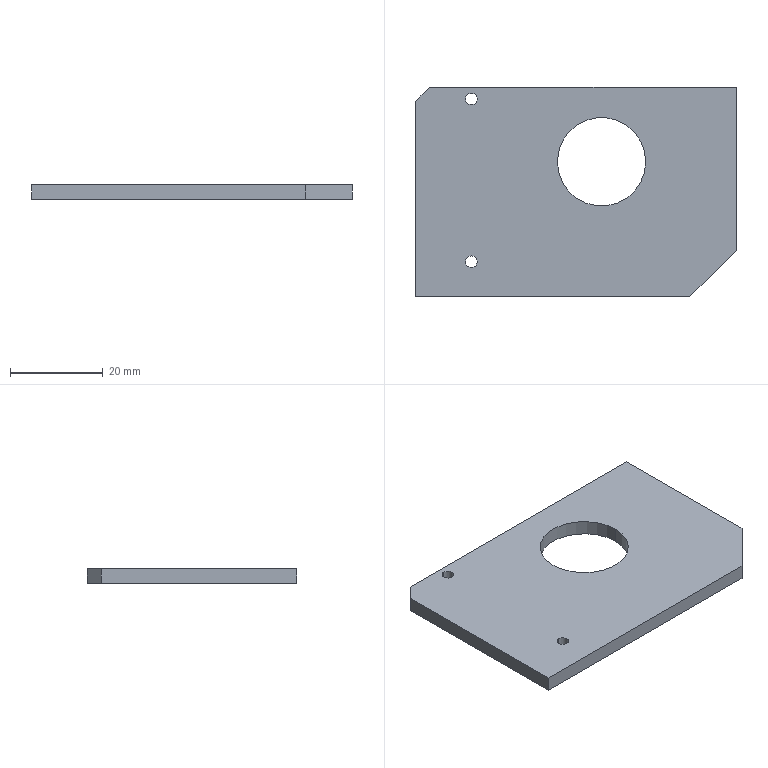Part | STEP file | [02]-14 | 1 solid | 14 faces | box 69 x 45 x 3.2 mm | volume 8823 mm3 | plane 8 | cylinder 6 | commonest cylinder face diameters 2.5 x4 19 x2
STEP:
#1=CARTESIAN_POINT('',(0.,0.,0.));
#2=DIRECTION('',(0.,0.,1.));
#3=DIRECTION('',(1.,0.,0.));
#4=AXIS2_PLACEMENT_3D('',#1,#2,#3);
#5=CARTESIAN_POINT('',(12.,-38.75,3.));
#6=VERTEX_POINT('',#5);
#7=CARTESIAN_POINT('',(12.,-38.75,-0.2));
#8=VERTEX_POINT('',#7);
#9=CARTESIAN_POINT('',(12.,-38.75,3.));
#10=DIRECTION('',(0.,0.,-1.));
#11=VECTOR('',#10,1.);
#12=LINE('',#9,#11);
#13=CARTESIAN_POINT('',(12.,-37.5,3.));
#14=DIRECTION('',(0.,0.,-1.));
#15=DIRECTION('',(0.,-1.,0.));
#16=AXIS2_PLACEMENT_3D('',#13,#14,#15);
#17=CYLINDRICAL_SURFACE('',#16,1.25);
#18=CARTESIAN_POINT('',(6.283,0.));
#19=DIRECTION('',(0.,1.));
#20=VECTOR('',#19,1.);
#21=LINE('',#18,#20);
#22=(GEOMETRIC_REPRESENTATION_CONTEXT(2)PARAMETRIC_REPRESENTATION_CONTEXT()REPRESENTATION_CONTEXT('',''));
#23=DEFINITIONAL_REPRESENTATION('',(#21),#22);
#24=PCURVE('',#17,#23);
#25=CARTESIAN_POINT('',(12.,-37.5,3.));
#26=DIRECTION('',(0.,0.,-1.));
#27=DIRECTION('',(0.,-1.,0.));
#28=AXIS2_PLACEMENT_3D('',#25,#26,#27);
#29=CYLINDRICAL_SURFACE('',#28,1.25);
#30=CARTESIAN_POINT('',(0.,0.));
#31=DIRECTION('',(0.,1.));
#32=VECTOR('',#31,1.);
#33=LINE('',#30,#32);
#34=(GEOMETRIC_REPRESENTATION_CONTEXT(2)PARAMETRIC_REPRESENTATION_CONTEXT()REPRESENTATION_CONTEXT('',''));
#35=DEFINITIONAL_REPRESENTATION('',(#33),#34);
#36=PCURVE('',#29,#35);
#37=SURFACE_CURVE('',#12,(#24,#36),.PCURVE_S1.);
#38=EDGE_CURVE('',#6,#8,#37,.T.);
#39=ORIENTED_EDGE('',*,*,#38,.T.);
#40=CARTESIAN_POINT('',(12.,-36.25,-0.2));
#41=VERTEX_POINT('',#40);
#42=CARTESIAN_POINT('',(12.,-37.5,-0.2));
#43=DIRECTION('',(0.,0.,1.));
#44=DIRECTION('',(0.,1.,0.));
#45=AXIS2_PLACEMENT_3D('',#42,#43,#44);
#46=CIRCLE('',#45,1.25);
#47=CARTESIAN_POINT('',(9.425,3.2));
#48=DIRECTION('',(-1.,0.));
#49=VECTOR('',#48,1.);
#50=LINE('',#47,#49);
#51=(GEOMETRIC_REPRESENTATION_CONTEXT(2)PARAMETRIC_REPRESENTATION_CONTEXT()REPRESENTATION_CONTEXT('',''));
#52=DEFINITIONAL_REPRESENTATION('',(#50),#51);
#53=PCURVE('',#17,#52);
#54=CARTESIAN_POINT('',(34.5,-22.5,-0.2));
#55=DIRECTION('',(0.,0.,-1.));
#56=DIRECTION('',(0.,-1.,0.));
#57=AXIS2_PLACEMENT_3D('',#54,#55,#56);
#58=PLANE('',#57);
#59=CARTESIAN_POINT('',(13.75,22.5));
#60=CARTESIAN_POINT('',(13.75,24.665));
#61=CARTESIAN_POINT('',(15.625,23.583));
#62=CARTESIAN_POINT('',(17.5,22.5));
#63=CARTESIAN_POINT('',(15.625,21.417));
#64=CARTESIAN_POINT('',(13.75,20.335));
#65=CARTESIAN_POINT('',(13.75,22.5));
#66=(BOUNDED_CURVE()B_SPLINE_CURVE(2,(#59,#60,#61,#62,#63,#64,#65),.UNSPECIFIED.,.T.,.F.)B_SPLINE_CURVE_WITH_KNOTS((1,2,2,2,2,1),(-2.094,0.,2.094,4.189,6.283,8.378),.UNSPECIFIED.)CURVE()GEOMETRIC_REPRESENTATION_ITEM()RATIONAL_B_SPLINE_CURVE((1.,0.5,1.,0.5,1.,0.5,1.))REPRESENTATION_ITEM(''));
#67=(GEOMETRIC_REPRESENTATION_CONTEXT(2)PARAMETRIC_REPRESENTATION_CONTEXT()REPRESENTATION_CONTEXT('',''));
#68=DEFINITIONAL_REPRESENTATION('',(#66),#67);
#69=PCURVE('',#58,#68);
#70=SURFACE_CURVE('',#46,(#53,#69),.PCURVE_S1.);
#71=EDGE_CURVE('',#8,#41,#70,.T.);
#72=ORIENTED_EDGE('',*,*,#71,.T.);
#73=CARTESIAN_POINT('',(12.,-36.25,3.));
#74=VERTEX_POINT('',#73);
#75=CARTESIAN_POINT('',(12.,-36.25,3.));
#76=DIRECTION('',(0.,0.,-1.));
#77=VECTOR('',#76,1.);
#78=LINE('',#75,#77);
#79=CARTESIAN_POINT('',(3.142,0.));
#80=DIRECTION('',(0.,1.));
#81=VECTOR('',#80,1.);
#82=LINE('',#79,#81);
#83=(GEOMETRIC_REPRESENTATION_CONTEXT(2)PARAMETRIC_REPRESENTATION_CONTEXT()REPRESENTATION_CONTEXT('',''));
#84=DEFINITIONAL_REPRESENTATION('',(#82),#83);
#85=PCURVE('',#17,#84);
#86=CARTESIAN_POINT('',(3.142,0.));
#87=DIRECTION('',(0.,1.));
#88=VECTOR('',#87,1.);
#89=LINE('',#86,#88);
#90=(GEOMETRIC_REPRESENTATION_CONTEXT(2)PARAMETRIC_REPRESENTATION_CONTEXT()REPRESENTATION_CONTEXT('',''));
#91=DEFINITIONAL_REPRESENTATION('',(#89),#90);
#92=PCURVE('',#29,#91);
#93=SURFACE_CURVE('',#78,(#85,#92),.PCURVE_S1.);
#94=EDGE_CURVE('',#74,#41,#93,.T.);
#95=ORIENTED_EDGE('',*,*,#94,.F.);
#96=CARTESIAN_POINT('',(12.,-37.5,3.));
#97=DIRECTION('',(0.,0.,-1.));
#98=DIRECTION('',(0.,-1.,0.));
#99=AXIS2_PLACEMENT_3D('',#96,#97,#98);
#100=CIRCLE('',#99,1.25);
#101=CARTESIAN_POINT('',(0.,0.));
#102=DIRECTION('',(1.,0.));
#103=VECTOR('',#102,1.);
#104=LINE('',#101,#103);
#105=(GEOMETRIC_REPRESENTATION_CONTEXT(2)PARAMETRIC_REPRESENTATION_CONTEXT()REPRESENTATION_CONTEXT('',''));
#106=DEFINITIONAL_REPRESENTATION('',(#104),#105);
#107=PCURVE('',#17,#106);
#108=CARTESIAN_POINT('',(34.5,-22.5,3.));
#109=DIRECTION('',(0.,0.,1.));
#110=DIRECTION('',(0.,1.,0.));
#111=AXIS2_PLACEMENT_3D('',#108,#109,#110);
#112=PLANE('',#111);
#113=CARTESIAN_POINT('',(-16.25,22.5));
#114=CARTESIAN_POINT('',(-16.25,24.665));
#115=CARTESIAN_POINT('',(-14.375,23.583));
#116=CARTESIAN_POINT('',(-12.5,22.5));
#117=CARTESIAN_POINT('',(-14.375,21.417));
#118=CARTESIAN_POINT('',(-16.25,20.335));
#119=CARTESIAN_POINT('',(-16.25,22.5));
#120=(BOUNDED_CURVE()B_SPLINE_CURVE(2,(#113,#114,#115,#116,#117,#118,#119),.UNSPECIFIED.,.T.,.F.)B_SPLINE_CURVE_WITH_KNOTS((1,2,2,2,2,1),(-2.094,0.,2.094,4.189,6.283,8.378),.UNSPECIFIED.)CURVE()GEOMETRIC_REPRESENTATION_ITEM()RATIONAL_B_SPLINE_CURVE((1.,0.5,1.,0.5,1.,0.5,1.))REPRESENTATION_ITEM(''));
#121=(GEOMETRIC_REPRESENTATION_CONTEXT(2)PARAMETRIC_REPRESENTATION_CONTEXT()REPRESENTATION_CONTEXT('',''));
#122=DEFINITIONAL_REPRESENTATION('',(#120),#121);
#123=PCURVE('',#112,#122);
#124=SURFACE_CURVE('',#100,(#107,#123),.PCURVE_S1.);
#125=EDGE_CURVE('',#74,#6,#124,.T.);
#126=ORIENTED_EDGE('',*,*,#125,.T.);
#127=EDGE_LOOP('',(#39,#72,#95,#126));
#128=FACE_BOUND('',#127,.F.);
#129=ADVANCED_FACE('',(#128),#17,.F.);
#130=CARTESIAN_POINT('',(12.,-3.75,3.));
#131=VERTEX_POINT('',#130);
#132=CARTESIAN_POINT('',(12.,-3.75,-0.2));
#133=VERTEX_POINT('',#132);
#134=CARTESIAN_POINT('',(12.,-3.75,3.));
#135=DIRECTION('',(0.,0.,-1.));
#136=VECTOR('',#135,1.);
#137=LINE('',#134,#136);
#138=CARTESIAN_POINT('',(12.,-2.5,3.));
#139=DIRECTION('',(0.,0.,-1.));
#140=DIRECTION('',(0.,-1.,0.));
#141=AXIS2_PLACEMENT_3D('',#138,#139,#140);
#142=CYLINDRICAL_SURFACE('',#141,1.25);
#143=CARTESIAN_POINT('',(6.283,0.));
#144=DIRECTION('',(0.,1.));
#145=VECTOR('',#144,1.);
#146=LINE('',#143,#145);
#147=(GEOMETRIC_REPRESENTATION_CONTEXT(2)PARAMETRIC_REPRESENTATION_CONTEXT()REPRESENTATION_CONTEXT('',''));
#148=DEFINITIONAL_REPRESENTATION('',(#146),#147);
#149=PCURVE('',#142,#148);
#150=CARTESIAN_POINT('',(12.,-2.5,3.));
#151=DIRECTION('',(0.,0.,-1.));
#152=DIRECTION('',(0.,-1.,0.));
#153=AXIS2_PLACEMENT_3D('',#150,#151,#152);
#154=CYLINDRICAL_SURFACE('',#153,1.25);
#155=CARTESIAN_POINT('',(0.,0.));
#156=DIRECTION('',(0.,1.));
#157=VECTOR('',#156,1.);
#158=LINE('',#155,#157);
#159=(GEOMETRIC_REPRESENTATION_CONTEXT(2)PARAMETRIC_REPRESENTATION_CONTEXT()REPRESENTATION_CONTEXT('',''));
#160=DEFINITIONAL_REPRESENTATION('',(#158),#159);
#161=PCURVE('',#154,#160);
#162=SURFACE_CURVE('',#137,(#149,#161),.PCURVE_S1.);
#163=EDGE_CURVE('',#131,#133,#162,.T.);
#164=ORIENTED_EDGE('',*,*,#163,.T.);
#165=CARTESIAN_POINT('',(12.,-1.25,-0.2));
#166=VERTEX_POINT('',#165);
#167=CARTESIAN_POINT('',(12.,-2.5,-0.2));
#168=DIRECTION('',(0.,0.,1.));
#169=DIRECTION('',(0.,1.,0.));
#170=AXIS2_PLACEMENT_3D('',#167,#168,#169);
#171=CIRCLE('',#170,1.25);
#172=CARTESIAN_POINT('',(9.425,3.2));
#173=DIRECTION('',(-1.,0.));
#174=VECTOR('',#173,1.);
#175=LINE('',#172,#174);
#176=(GEOMETRIC_REPRESENTATION_CONTEXT(2)PARAMETRIC_REPRESENTATION_CONTEXT()REPRESENTATION_CONTEXT('',''));
#177=DEFINITIONAL_REPRESENTATION('',(#175),#176);
#178=PCURVE('',#142,#177);
#179=CARTESIAN_POINT('',(-21.25,22.5));
#180=CARTESIAN_POINT('',(-21.25,24.665));
#181=CARTESIAN_POINT('',(-19.375,23.583));
#182=CARTESIAN_POINT('',(-17.5,22.5));
#183=CARTESIAN_POINT('',(-19.375,21.417));
#184=CARTESIAN_POINT('',(-21.25,20.335));
#185=CARTESIAN_POINT('',(-21.25,22.5));
#186=(BOUNDED_CURVE()B_SPLINE_CURVE(2,(#179,#180,#181,#182,#183,#184,#185),.UNSPECIFIED.,.T.,.F.)B_SPLINE_CURVE_WITH_KNOTS((1,2,2,2,2,1),(-2.094,0.,2.094,4.189,6.283,8.378),.UNSPECIFIED.)CURVE()GEOMETRIC_REPRESENTATION_ITEM()RATIONAL_B_SPLINE_CURVE((1.,0.5,1.,0.5,1.,0.5,1.))REPRESENTATION_ITEM(''));
#187=(GEOMETRIC_REPRESENTATION_CONTEXT(2)PARAMETRIC_REPRESENTATION_CONTEXT()REPRESENTATION_CONTEXT('',''));
#188=DEFINITIONAL_REPRESENTATION('',(#186),#187);
#189=PCURVE('',#58,#188);
#190=SURFACE_CURVE('',#171,(#178,#189),.PCURVE_S1.);
#191=EDGE_CURVE('',#133,#166,#190,.T.);
#192=ORIENTED_EDGE('',*,*,#191,.T.);
#193=CARTESIAN_POINT('',(12.,-1.25,3.));
#194=VERTEX_POINT('',#193);
#195=CARTESIAN_POINT('',(12.,-1.25,3.));
#196=DIRECTION('',(0.,0.,-1.));
#197=VECTOR('',#196,1.);
#198=LINE('',#195,#197);
#199=CARTESIAN_POINT('',(3.142,0.));
#200=DIRECTION('',(0.,1.));
#201=VECTOR('',#200,1.);
#202=LINE('',#199,#201);
#203=(GEOMETRIC_REPRESENTATION_CONTEXT(2)PARAMETRIC_REPRESENTATION_CONTEXT()REPRESENTATION_CONTEXT('',''));
#204=DEFINITIONAL_REPRESENTATION('',(#202),#203);
#205=PCURVE('',#142,#204);
#206=CARTESIAN_POINT('',(3.142,0.));
#207=DIRECTION('',(0.,1.));
#208=VECTOR('',#207,1.);
#209=LINE('',#206,#208);
#210=(GEOMETRIC_REPRESENTATION_CONTEXT(2)PARAMETRIC_REPRESENTATION_CONTEXT()REPRESENTATION_CONTEXT('',''));
#211=DEFINITIONAL_REPRESENTATION('',(#209),#210);
#212=PCURVE('',#154,#211);
#213=SURFACE_CURVE('',#198,(#205,#212),.PCURVE_S1.);
#214=EDGE_CURVE('',#194,#166,#213,.T.);
#215=ORIENTED_EDGE('',*,*,#214,.F.);
#216=CARTESIAN_POINT('',(12.,-2.5,3.));
#217=DIRECTION('',(0.,0.,-1.));
#218=DIRECTION('',(0.,-1.,0.));
#219=AXIS2_PLACEMENT_3D('',#216,#217,#218);
#220=CIRCLE('',#219,1.25);
#221=CARTESIAN_POINT('',(0.,0.));
#222=DIRECTION('',(1.,0.));
#223=VECTOR('',#222,1.);
#224=LINE('',#221,#223);
#225=(GEOMETRIC_REPRESENTATION_CONTEXT(2)PARAMETRIC_REPRESENTATION_CONTEXT()REPRESENTATION_CONTEXT('',''));
#226=DEFINITIONAL_REPRESENTATION('',(#224),#225);
#227=PCURVE('',#142,#226);
#228=CARTESIAN_POINT('',(18.75,22.5));
#229=CARTESIAN_POINT('',(18.75,24.665));
#230=CARTESIAN_POINT('',(20.625,23.583));
#231=CARTESIAN_POINT('',(22.5,22.5));
#232=CARTESIAN_POINT('',(20.625,21.417));
#233=CARTESIAN_POINT('',(18.75,20.335));
#234=CARTESIAN_POINT('',(18.75,22.5));
#235=(BOUNDED_CURVE()B_SPLINE_CURVE(2,(#228,#229,#230,#231,#232,#233,#234),.UNSPECIFIED.,.T.,.F.)B_SPLINE_CURVE_WITH_KNOTS((1,2,2,2,2,1),(-2.094,0.,2.094,4.189,6.283,8.378),.UNSPECIFIED.)CURVE()GEOMETRIC_REPRESENTATION_ITEM()RATIONAL_B_SPLINE_CURVE((1.,0.5,1.,0.5,1.,0.5,1.))REPRESENTATION_ITEM(''));
#236=(GEOMETRIC_REPRESENTATION_CONTEXT(2)PARAMETRIC_REPRESENTATION_CONTEXT()REPRESENTATION_CONTEXT('',''));
#237=DEFINITIONAL_REPRESENTATION('',(#235),#236);
#238=PCURVE('',#112,#237);
#239=SURFACE_CURVE('',#220,(#227,#238),.PCURVE_S1.);
#240=EDGE_CURVE('',#194,#131,#239,.T.);
#241=ORIENTED_EDGE('',*,*,#240,.T.);
#242=EDGE_LOOP('',(#164,#192,#215,#241));
#243=FACE_BOUND('',#242,.F.);
#244=ADVANCED_FACE('',(#243),#142,.F.);
#245=CARTESIAN_POINT('',(49.5,-16.,-0.2));
#246=VERTEX_POINT('',#245);
#247=CARTESIAN_POINT('',(49.5,-16.,3.));
#248=VERTEX_POINT('',#247);
#249=CARTESIAN_POINT('',(49.5,-16.,-0.2));
#250=DIRECTION('',(0.,0.,1.));
#251=VECTOR('',#250,1.);
#252=LINE('',#249,#251);
#253=CARTESIAN_POINT('',(40.,-16.,-0.2));
#254=DIRECTION('',(0.,0.,1.));
#255=DIRECTION('',(1.,0.,0.));
#256=AXIS2_PLACEMENT_3D('',#253,#254,#255);
#257=CYLINDRICAL_SURFACE('',#256,9.5);
#258=CARTESIAN_POINT('',(6.283,0.));
#259=DIRECTION('',(0.,1.));
#260=VECTOR('',#259,1.);
#261=LINE('',#258,#260);
#262=(GEOMETRIC_REPRESENTATION_CONTEXT(2)PARAMETRIC_REPRESENTATION_CONTEXT()REPRESENTATION_CONTEXT('',''));
#263=DEFINITIONAL_REPRESENTATION('',(#261),#262);
#264=PCURVE('',#257,#263);
#265=CARTESIAN_POINT('',(40.,-16.,-0.2));
#266=DIRECTION('',(0.,0.,1.));
#267=DIRECTION('',(1.,0.,0.));
#268=AXIS2_PLACEMENT_3D('',#265,#266,#267);
#269=CYLINDRICAL_SURFACE('',#268,9.5);
#270=CARTESIAN_POINT('',(0.,0.));
#271=DIRECTION('',(0.,1.));
#272=VECTOR('',#271,1.);
#273=LINE('',#270,#272);
#274=(GEOMETRIC_REPRESENTATION_CONTEXT(2)PARAMETRIC_REPRESENTATION_CONTEXT()REPRESENTATION_CONTEXT('',''));
#275=DEFINITIONAL_REPRESENTATION('',(#273),#274);
#276=PCURVE('',#269,#275);
#277=SURFACE_CURVE('',#252,(#264,#276),.PCURVE_S1.);
#278=EDGE_CURVE('',#246,#248,#277,.T.);
#279=ORIENTED_EDGE('',*,*,#278,.T.);
#280=CARTESIAN_POINT('',(30.5,-16.,3.));
#281=VERTEX_POINT('',#280);
#282=CARTESIAN_POINT('',(40.,-16.,3.));
#283=DIRECTION('',(0.,0.,1.));
#284=DIRECTION('',(-1.,0.,0.));
#285=AXIS2_PLACEMENT_3D('',#282,#283,#284);
#286=CIRCLE('',#285,9.5);
#287=CARTESIAN_POINT('',(3.142,3.2));
#288=DIRECTION('',(1.,0.));
#289=VECTOR('',#288,1.);
#290=LINE('',#287,#289);
#291=(GEOMETRIC_REPRESENTATION_CONTEXT(2)PARAMETRIC_REPRESENTATION_CONTEXT()REPRESENTATION_CONTEXT('',''));
#292=DEFINITIONAL_REPRESENTATION('',(#290),#291);
#293=PCURVE('',#257,#292);
#294=CARTESIAN_POINT('',(6.5,-5.5));
#295=DIRECTION('',(0.,1.));
#296=AXIS2_PLACEMENT_2D('',#294,#295);
#297=CIRCLE('',#296,9.5);
#298=(GEOMETRIC_REPRESENTATION_CONTEXT(2)PARAMETRIC_REPRESENTATION_CONTEXT()REPRESENTATION_CONTEXT('',''));
#299=DEFINITIONAL_REPRESENTATION('',(#297),#298);
#300=PCURVE('',#112,#299);
#301=SURFACE_CURVE('',#286,(#293,#300),.PCURVE_S1.);
#302=EDGE_CURVE('',#281,#248,#301,.T.);
#303=ORIENTED_EDGE('',*,*,#302,.F.);
#304=CARTESIAN_POINT('',(30.5,-16.,-0.2));
#305=VERTEX_POINT('',#304);
#306=CARTESIAN_POINT('',(30.5,-16.,-0.2));
#307=DIRECTION('',(0.,0.,1.));
#308=VECTOR('',#307,1.);
#309=LINE('',#306,#308);
#310=CARTESIAN_POINT('',(3.142,0.));
#311=DIRECTION('',(0.,1.));
#312=VECTOR('',#311,1.);
#313=LINE('',#310,#312);
#314=(GEOMETRIC_REPRESENTATION_CONTEXT(2)PARAMETRIC_REPRESENTATION_CONTEXT()REPRESENTATION_CONTEXT('',''));
#315=DEFINITIONAL_REPRESENTATION('',(#313),#314);
#316=PCURVE('',#257,#315);
#317=CARTESIAN_POINT('',(3.142,0.));
#318=DIRECTION('',(0.,1.));
#319=VECTOR('',#318,1.);
#320=LINE('',#317,#319);
#321=(GEOMETRIC_REPRESENTATION_CONTEXT(2)PARAMETRIC_REPRESENTATION_CONTEXT()REPRESENTATION_CONTEXT('',''));
#322=DEFINITIONAL_REPRESENTATION('',(#320),#321);
#323=PCURVE('',#269,#322);
#324=SURFACE_CURVE('',#309,(#316,#323),.PCURVE_S1.);
#325=EDGE_CURVE('',#305,#281,#324,.T.);
#326=ORIENTED_EDGE('',*,*,#325,.F.);
#327=CARTESIAN_POINT('',(40.,-16.,-0.2));
#328=DIRECTION('',(0.,0.,-1.));
#329=DIRECTION('',(1.,0.,0.));
#330=AXIS2_PLACEMENT_3D('',#327,#328,#329);
#331=CIRCLE('',#330,9.5);
#332=CARTESIAN_POINT('',(6.283,0.));
#333=DIRECTION('',(-1.,0.));
#334=VECTOR('',#333,1.);
#335=LINE('',#332,#334);
#336=(GEOMETRIC_REPRESENTATION_CONTEXT(2)PARAMETRIC_REPRESENTATION_CONTEXT()REPRESENTATION_CONTEXT('',''));
#337=DEFINITIONAL_REPRESENTATION('',(#335),#336);
#338=PCURVE('',#257,#337);
#339=CARTESIAN_POINT('',(-6.5,-5.5));
#340=DIRECTION('',(0.,-1.));
#341=AXIS2_PLACEMENT_2D('',#339,#340);
#342=CIRCLE('',#341,9.5);
#343=(GEOMETRIC_REPRESENTATION_CONTEXT(2)PARAMETRIC_REPRESENTATION_CONTEXT()REPRESENTATION_CONTEXT('',''));
#344=DEFINITIONAL_REPRESENTATION('',(#342),#343);
#345=PCURVE('',#58,#344);
#346=SURFACE_CURVE('',#331,(#338,#345),.PCURVE_S1.);
#347=EDGE_CURVE('',#246,#305,#346,.T.);
#348=ORIENTED_EDGE('',*,*,#347,.F.);
#349=EDGE_LOOP('',(#279,#303,#326,#348));
#350=FACE_BOUND('',#349,.F.);
#351=ADVANCED_FACE('',(#350),#257,.F.);
#352=CARTESIAN_POINT('',(12.,-37.5,3.));
#353=DIRECTION('',(0.,0.,-1.));
#354=DIRECTION('',(0.,-1.,0.));
#355=AXIS2_PLACEMENT_3D('',#352,#353,#354);
#356=CIRCLE('',#355,1.25);
#357=CARTESIAN_POINT('',(-16.25,22.5));
#358=CARTESIAN_POINT('',(-16.25,24.665));
#359=CARTESIAN_POINT('',(-14.375,23.583));
#360=CARTESIAN_POINT('',(-12.5,22.5));
#361=CARTESIAN_POINT('',(-14.375,21.417));
#362=CARTESIAN_POINT('',(-16.25,20.335));
#363=CARTESIAN_POINT('',(-16.25,22.5));
#364=(BOUNDED_CURVE()B_SPLINE_CURVE(2,(#357,#358,#359,#360,#361,#362,#363),.UNSPECIFIED.,.T.,.F.)B_SPLINE_CURVE_WITH_KNOTS((1,2,2,2,2,1),(-2.094,0.,2.094,4.189,6.283,8.378),.UNSPECIFIED.)CURVE()GEOMETRIC_REPRESENTATION_ITEM()RATIONAL_B_SPLINE_CURVE((1.,0.5,1.,0.5,1.,0.5,1.))REPRESENTATION_ITEM(''));
#365=(GEOMETRIC_REPRESENTATION_CONTEXT(2)PARAMETRIC_REPRESENTATION_CONTEXT()REPRESENTATION_CONTEXT('',''));
#366=DEFINITIONAL_REPRESENTATION('',(#364),#365);
#367=PCURVE('',#112,#366);
#368=CARTESIAN_POINT('',(0.,0.));
#369=DIRECTION('',(1.,0.));
#370=VECTOR('',#369,1.);
#371=LINE('',#368,#370);
#372=(GEOMETRIC_REPRESENTATION_CONTEXT(2)PARAMETRIC_REPRESENTATION_CONTEXT()REPRESENTATION_CONTEXT('',''));
#373=DEFINITIONAL_REPRESENTATION('',(#371),#372);
#374=PCURVE('',#29,#373);
#375=SURFACE_CURVE('',#356,(#367,#374),.PCURVE_S1.);
#376=EDGE_CURVE('',#6,#74,#375,.T.);
#377=ORIENTED_EDGE('',*,*,#376,.T.);
#378=ORIENTED_EDGE('',*,*,#125,.T.);
#379=EDGE_LOOP('',(#377,#378));
#380=FACE_BOUND('',#379,.T.);
#381=CARTESIAN_POINT('',(12.,-2.5,3.));
#382=DIRECTION('',(0.,0.,-1.));
#383=DIRECTION('',(0.,-1.,0.));
#384=AXIS2_PLACEMENT_3D('',#381,#382,#383);
#385=CIRCLE('',#384,1.25);
#386=CARTESIAN_POINT('',(18.75,22.5));
#387=CARTESIAN_POINT('',(18.75,24.665));
#388=CARTESIAN_POINT('',(20.625,23.583));
#389=CARTESIAN_POINT('',(22.5,22.5));
#390=CARTESIAN_POINT('',(20.625,21.417));
#391=CARTESIAN_POINT('',(18.75,20.335));
#392=CARTESIAN_POINT('',(18.75,22.5));
#393=(BOUNDED_CURVE()B_SPLINE_CURVE(2,(#386,#387,#388,#389,#390,#391,#392),.UNSPECIFIED.,.T.,.F.)B_SPLINE_CURVE_WITH_KNOTS((1,2,2,2,2,1),(-2.094,0.,2.094,4.189,6.283,8.378),.UNSPECIFIED.)CURVE()GEOMETRIC_REPRESENTATION_ITEM()RATIONAL_B_SPLINE_CURVE((1.,0.5,1.,0.5,1.,0.5,1.))REPRESENTATION_ITEM(''));
#394=(GEOMETRIC_REPRESENTATION_CONTEXT(2)PARAMETRIC_REPRESENTATION_CONTEXT()REPRESENTATION_CONTEXT('',''));
#395=DEFINITIONAL_REPRESENTATION('',(#393),#394);
#396=PCURVE('',#112,#395);
#397=CARTESIAN_POINT('',(0.,0.));
#398=DIRECTION('',(1.,0.));
#399=VECTOR('',#398,1.);
#400=LINE('',#397,#399);
#401=(GEOMETRIC_REPRESENTATION_CONTEXT(2)PARAMETRIC_REPRESENTATION_CONTEXT()REPRESENTATION_CONTEXT('',''));
#402=DEFINITIONAL_REPRESENTATION('',(#400),#401);
#403=PCURVE('',#154,#402);
#404=SURFACE_CURVE('',#385,(#396,#403),.PCURVE_S1.);
#405=EDGE_CURVE('',#131,#194,#404,.T.);
#406=ORIENTED_EDGE('',*,*,#405,.T.);
#407=ORIENTED_EDGE('',*,*,#240,.T.);
#408=EDGE_LOOP('',(#406,#407));
#409=FACE_BOUND('',#408,.T.);
#410=CARTESIAN_POINT('',(40.,-16.,3.));
#411=DIRECTION('',(0.,0.,1.));
#412=DIRECTION('',(-1.,0.,0.));
#413=AXIS2_PLACEMENT_3D('',#410,#411,#412);
#414=CIRCLE('',#413,9.5);
#415=CARTESIAN_POINT('',(6.5,-5.5));
#416=DIRECTION('',(0.,1.));
#417=AXIS2_PLACEMENT_2D('',#415,#416);
#418=CIRCLE('',#417,9.5);
#419=(GEOMETRIC_REPRESENTATION_CONTEXT(2)PARAMETRIC_REPRESENTATION_CONTEXT()REPRESENTATION_CONTEXT('',''));
#420=DEFINITIONAL_REPRESENTATION('',(#418),#419);
#421=PCURVE('',#112,#420);
#422=CARTESIAN_POINT('',(-3.142,3.2));
#423=DIRECTION('',(1.,0.));
#424=VECTOR('',#423,1.);
#425=LINE('',#422,#424);
#426=(GEOMETRIC_REPRESENTATION_CONTEXT(2)PARAMETRIC_REPRESENTATION_CONTEXT()REPRESENTATION_CONTEXT('',''));
#427=DEFINITIONAL_REPRESENTATION('',(#425),#426);
#428=PCURVE('',#269,#427);
#429=SURFACE_CURVE('',#414,(#421,#428),.PCURVE_S1.);
#430=EDGE_CURVE('',#248,#281,#429,.T.);
#431=ORIENTED_EDGE('',*,*,#430,.F.);
#432=ORIENTED_EDGE('',*,*,#302,.F.);
#433=EDGE_LOOP('',(#431,#432));
#434=FACE_BOUND('',#433,.T.);
#435=CARTESIAN_POINT('',(0.,-3.,3.));
#436=VERTEX_POINT('',#435);
#437=CARTESIAN_POINT('',(0.,-45.,3.));
#438=VERTEX_POINT('',#437);
#439=CARTESIAN_POINT('',(0.,-22.5,3.));
#440=DIRECTION('',(0.,-1.,0.));
#441=VECTOR('',#440,1.);
#442=LINE('',#439,#441);
#443=CARTESIAN_POINT('',(0.,34.5));
#444=DIRECTION('',(-1.,0.));
#445=VECTOR('',#444,1.);
#446=LINE('',#443,#445);
#447=(GEOMETRIC_REPRESENTATION_CONTEXT(2)PARAMETRIC_REPRESENTATION_CONTEXT()REPRESENTATION_CONTEXT('',''));
#448=DEFINITIONAL_REPRESENTATION('',(#446),#447);
#449=PCURVE('',#112,#448);
#450=CARTESIAN_POINT('',(0.,-22.5,-0.2));
#451=DIRECTION('',(-1.,0.,0.));
#452=DIRECTION('',(0.,0.,-1.));
#453=AXIS2_PLACEMENT_3D('',#450,#451,#452);
#454=PLANE('',#453);
#455=CARTESIAN_POINT('',(-3.2,0.));
#456=DIRECTION('',(0.,1.));
#457=VECTOR('',#456,1.);
#458=LINE('',#455,#457);
#459=(GEOMETRIC_REPRESENTATION_CONTEXT(2)PARAMETRIC_REPRESENTATION_CONTEXT()REPRESENTATION_CONTEXT('',''));
#460=DEFINITIONAL_REPRESENTATION('',(#458),#459);
#461=PCURVE('',#454,#460);
#462=SURFACE_CURVE('',#442,(#449,#461),.PCURVE_S1.);
#463=EDGE_CURVE('',#436,#438,#462,.T.);
#464=ORIENTED_EDGE('',*,*,#463,.T.);
#465=CARTESIAN_POINT('',(59.,-45.,3.));
#466=VERTEX_POINT('',#465);
#467=CARTESIAN_POINT('',(34.5,-45.,3.));
#468=DIRECTION('',(1.,0.,0.));
#469=VECTOR('',#468,1.);
#470=LINE('',#467,#469);
#471=CARTESIAN_POINT('',(-22.5,0.));
#472=DIRECTION('',(0.,-1.));
#473=VECTOR('',#472,1.);
#474=LINE('',#471,#473);
#475=(GEOMETRIC_REPRESENTATION_CONTEXT(2)PARAMETRIC_REPRESENTATION_CONTEXT()REPRESENTATION_CONTEXT('',''));
#476=DEFINITIONAL_REPRESENTATION('',(#474),#475);
#477=PCURVE('',#112,#476);
#478=CARTESIAN_POINT('',(34.5,-45.,-0.2));
#479=DIRECTION('',(0.,-1.,0.));
#480=DIRECTION('',(0.,0.,1.));
#481=AXIS2_PLACEMENT_3D('',#478,#479,#480);
#482=PLANE('',#481);
#483=CARTESIAN_POINT('',(3.2,0.));
#484=DIRECTION('',(0.,-1.));
#485=VECTOR('',#484,1.);
#486=LINE('',#483,#485);
#487=(GEOMETRIC_REPRESENTATION_CONTEXT(2)PARAMETRIC_REPRESENTATION_CONTEXT()REPRESENTATION_CONTEXT('',''));
#488=DEFINITIONAL_REPRESENTATION('',(#486),#487);
#489=PCURVE('',#482,#488);
#490=SURFACE_CURVE('',#470,(#477,#489),.PCURVE_S1.);
#491=EDGE_CURVE('',#438,#466,#490,.T.);
#492=ORIENTED_EDGE('',*,*,#491,.T.);
#493=CARTESIAN_POINT('',(69.,-35.,3.));
#494=VERTEX_POINT('',#493);
#495=CARTESIAN_POINT('',(58.,-46.,3.));
#496=DIRECTION('',(-0.7071,-0.7071,0.));
#497=VECTOR('',#496,1.);
#498=LINE('',#495,#497);
#499=CARTESIAN_POINT('',(-23.5,-23.5));
#500=DIRECTION('',(-0.7071,0.7071));
#501=VECTOR('',#500,1.);
#502=LINE('',#499,#501);
#503=(GEOMETRIC_REPRESENTATION_CONTEXT(2)PARAMETRIC_REPRESENTATION_CONTEXT()REPRESENTATION_CONTEXT('',''));
#504=DEFINITIONAL_REPRESENTATION('',(#502),#503);
#505=PCURVE('',#112,#504);
#506=CARTESIAN_POINT('',(69.,-35.,-0.2));
#507=DIRECTION('',(-0.7071,0.7071,0.));
#508=DIRECTION('',(0.,0.,1.));
#509=AXIS2_PLACEMENT_3D('',#506,#507,#508);
#510=PLANE('',#509);
#511=CARTESIAN_POINT('',(3.2,-15.556));
#512=DIRECTION('',(0.,-1.));
#513=VECTOR('',#512,1.);
#514=LINE('',#511,#513);
#515=(GEOMETRIC_REPRESENTATION_CONTEXT(2)PARAMETRIC_REPRESENTATION_CONTEXT()REPRESENTATION_CONTEXT('',''));
#516=DEFINITIONAL_REPRESENTATION('',(#514),#515);
#517=PCURVE('',#510,#516);
#518=SURFACE_CURVE('',#498,(#505,#517),.PCURVE_S1.);
#519=EDGE_CURVE('',#494,#466,#518,.T.);
#520=ORIENTED_EDGE('',*,*,#519,.F.);
#521=CARTESIAN_POINT('',(69.,0.,3.));
#522=VERTEX_POINT('',#521);
#523=CARTESIAN_POINT('',(69.,-22.5,3.));
#524=DIRECTION('',(0.,1.,0.));
#525=VECTOR('',#524,1.);
#526=LINE('',#523,#525);
#527=CARTESIAN_POINT('',(0.,-34.5));
#528=DIRECTION('',(1.,0.));
#529=VECTOR('',#528,1.);
#530=LINE('',#527,#529);
#531=(GEOMETRIC_REPRESENTATION_CONTEXT(2)PARAMETRIC_REPRESENTATION_CONTEXT()REPRESENTATION_CONTEXT('',''));
#532=DEFINITIONAL_REPRESENTATION('',(#530),#531);
#533=PCURVE('',#112,#532);
#534=CARTESIAN_POINT('',(69.,-22.5,-0.2));
#535=DIRECTION('',(1.,0.,0.));
#536=DIRECTION('',(0.,0.,1.));
#537=AXIS2_PLACEMENT_3D('',#534,#535,#536);
#538=PLANE('',#537);
#539=CARTESIAN_POINT('',(3.2,0.));
#540=DIRECTION('',(0.,-1.));
#541=VECTOR('',#540,1.);
#542=LINE('',#539,#541);
#543=(GEOMETRIC_REPRESENTATION_CONTEXT(2)PARAMETRIC_REPRESENTATION_CONTEXT()REPRESENTATION_CONTEXT('',''));
#544=DEFINITIONAL_REPRESENTATION('',(#542),#543);
#545=PCURVE('',#538,#544);
#546=SURFACE_CURVE('',#526,(#533,#545),.PCURVE_S1.);
#547=EDGE_CURVE('',#494,#522,#546,.T.);
#548=ORIENTED_EDGE('',*,*,#547,.T.);
#549=CARTESIAN_POINT('',(3.,0.,3.));
#550=VERTEX_POINT('',#549);
#551=CARTESIAN_POINT('',(34.5,0.,3.));
#552=DIRECTION('',(-1.,0.,0.));
#553=VECTOR('',#552,1.);
#554=LINE('',#551,#553);
#555=CARTESIAN_POINT('',(22.5,0.));
#556=DIRECTION('',(0.,1.));
#557=VECTOR('',#556,1.);
#558=LINE('',#555,#557);
#559=(GEOMETRIC_REPRESENTATION_CONTEXT(2)PARAMETRIC_REPRESENTATION_CONTEXT()REPRESENTATION_CONTEXT('',''));
#560=DEFINITIONAL_REPRESENTATION('',(#558),#559);
#561=PCURVE('',#112,#560);
#562=CARTESIAN_POINT('',(34.5,0.,-0.2));
#563=DIRECTION('',(0.,1.,0.));
#564=DIRECTION('',(0.,0.,-1.));
#565=AXIS2_PLACEMENT_3D('',#562,#563,#564);
#566=PLANE('',#565);
#567=CARTESIAN_POINT('',(-3.2,0.));
#568=DIRECTION('',(0.,1.));
#569=VECTOR('',#568,1.);
#570=LINE('',#567,#569);
#571=(GEOMETRIC_REPRESENTATION_CONTEXT(2)PARAMETRIC_REPRESENTATION_CONTEXT()REPRESENTATION_CONTEXT('',''));
#572=DEFINITIONAL_REPRESENTATION('',(#570),#571);
#573=PCURVE('',#566,#572);
#574=SURFACE_CURVE('',#554,(#561,#573),.PCURVE_S1.);
#575=EDGE_CURVE('',#522,#550,#574,.T.);
#576=ORIENTED_EDGE('',*,*,#575,.T.);
#577=CARTESIAN_POINT('',(7.5,4.5,3.));
#578=DIRECTION('',(0.7071,0.7071,0.));
#579=VECTOR('',#578,1.);
#580=LINE('',#577,#579);
#581=CARTESIAN_POINT('',(27.,27.));
#582=DIRECTION('',(0.7071,-0.7071));
#583=VECTOR('',#582,1.);
#584=LINE('',#581,#583);
#585=(GEOMETRIC_REPRESENTATION_CONTEXT(2)PARAMETRIC_REPRESENTATION_CONTEXT()REPRESENTATION_CONTEXT('',''));
#586=DEFINITIONAL_REPRESENTATION('',(#584),#585);
#587=PCURVE('',#112,#586);
#588=CARTESIAN_POINT('',(0.,-3.,-0.2));
#589=DIRECTION('',(0.7071,-0.7071,0.));
#590=DIRECTION('',(0.,0.,1.));
#591=AXIS2_PLACEMENT_3D('',#588,#589,#590);
#592=PLANE('',#591);
#593=CARTESIAN_POINT('',(3.2,-10.607));
#594=DIRECTION('',(0.,-1.));
#595=VECTOR('',#594,1.);
#596=LINE('',#593,#595);
#597=(GEOMETRIC_REPRESENTATION_CONTEXT(2)PARAMETRIC_REPRESENTATION_CONTEXT()REPRESENTATION_CONTEXT('',''));
#598=DEFINITIONAL_REPRESENTATION('',(#596),#597);
#599=PCURVE('',#592,#598);
#600=SURFACE_CURVE('',#580,(#587,#599),.PCURVE_S1.);
#601=EDGE_CURVE('',#436,#550,#600,.T.);
#602=ORIENTED_EDGE('',*,*,#601,.F.);
#603=EDGE_LOOP('',(#464,#492,#520,#548,#576,#602));
#604=FACE_BOUND('',#603,.T.);
#605=ADVANCED_FACE('',(#380,#409,#434,#604),#112,.T.);
#606=CARTESIAN_POINT('',(0.,-45.,-0.2));
#607=VERTEX_POINT('',#606);
#608=CARTESIAN_POINT('',(0.,-3.,-0.2));
#609=VERTEX_POINT('',#608);
#610=CARTESIAN_POINT('',(0.,-22.5,-0.2));
#611=DIRECTION('',(0.,1.,0.));
#612=VECTOR('',#611,1.);
#613=LINE('',#610,#612);
#614=CARTESIAN_POINT('',(0.,0.));
#615=DIRECTION('',(0.,-1.));
#616=VECTOR('',#615,1.);
#617=LINE('',#614,#616);
#618=(GEOMETRIC_REPRESENTATION_CONTEXT(2)PARAMETRIC_REPRESENTATION_CONTEXT()REPRESENTATION_CONTEXT('',''));
#619=DEFINITIONAL_REPRESENTATION('',(#617),#618);
#620=PCURVE('',#454,#619);
#621=CARTESIAN_POINT('',(0.,34.5));
#622=DIRECTION('',(-1.,0.));
#623=VECTOR('',#622,1.);
#624=LINE('',#621,#623);
#625=(GEOMETRIC_REPRESENTATION_CONTEXT(2)PARAMETRIC_REPRESENTATION_CONTEXT()REPRESENTATION_CONTEXT('',''));
#626=DEFINITIONAL_REPRESENTATION('',(#624),#625);
#627=PCURVE('',#58,#626);
#628=SURFACE_CURVE('',#613,(#620,#627),.PCURVE_S1.);
#629=EDGE_CURVE('',#607,#609,#628,.T.);
#630=ORIENTED_EDGE('',*,*,#629,.F.);
#631=CARTESIAN_POINT('',(0.,-45.,-0.2));
#632=DIRECTION('',(0.,0.,1.));
#633=VECTOR('',#632,1.);
#634=LINE('',#631,#633);
#635=CARTESIAN_POINT('',(0.,22.5));
#636=DIRECTION('',(-1.,0.));
#637=VECTOR('',#636,1.);
#638=LINE('',#635,#637);
#639=(GEOMETRIC_REPRESENTATION_CONTEXT(2)PARAMETRIC_REPRESENTATION_CONTEXT()REPRESENTATION_CONTEXT('',''));
#640=DEFINITIONAL_REPRESENTATION('',(#638),#639);
#641=PCURVE('',#454,#640);
#642=CARTESIAN_POINT('',(0.,34.5));
#643=DIRECTION('',(1.,0.));
#644=VECTOR('',#643,1.);
#645=LINE('',#642,#644);
#646=(GEOMETRIC_REPRESENTATION_CONTEXT(2)PARAMETRIC_REPRESENTATION_CONTEXT()REPRESENTATION_CONTEXT('',''));
#647=DEFINITIONAL_REPRESENTATION('',(#645),#646);
#648=PCURVE('',#482,#647);
#649=SURFACE_CURVE('',#634,(#641,#648),.PCURVE_S1.);
#650=EDGE_CURVE('',#607,#438,#649,.T.);
#651=ORIENTED_EDGE('',*,*,#650,.T.);
#652=ORIENTED_EDGE('',*,*,#463,.F.);
#653=CARTESIAN_POINT('',(0.,-3.,-0.2));
#654=DIRECTION('',(0.,0.,1.));
#655=VECTOR('',#654,1.);
#656=LINE('',#653,#655);
#657=CARTESIAN_POINT('',(0.,-19.5));
#658=DIRECTION('',(-1.,0.));
#659=VECTOR('',#658,1.);
#660=LINE('',#657,#659);
#661=(GEOMETRIC_REPRESENTATION_CONTEXT(2)PARAMETRIC_REPRESENTATION_CONTEXT()REPRESENTATION_CONTEXT('',''));
#662=DEFINITIONAL_REPRESENTATION('',(#660),#661);
#663=PCURVE('',#454,#662);
#664=CARTESIAN_POINT('',(0.,0.));
#665=DIRECTION('',(1.,0.));
#666=VECTOR('',#665,1.);
#667=LINE('',#664,#666);
#668=(GEOMETRIC_REPRESENTATION_CONTEXT(2)PARAMETRIC_REPRESENTATION_CONTEXT()REPRESENTATION_CONTEXT('',''));
#669=DEFINITIONAL_REPRESENTATION('',(#667),#668);
#670=PCURVE('',#592,#669);
#671=SURFACE_CURVE('',#656,(#663,#670),.PCURVE_S1.);
#672=EDGE_CURVE('',#609,#436,#671,.T.);
#673=ORIENTED_EDGE('',*,*,#672,.F.);
#674=EDGE_LOOP('',(#630,#651,#652,#673));
#675=FACE_BOUND('',#674,.T.);
#676=ADVANCED_FACE('',(#675),#454,.T.);
#677=ORIENTED_EDGE('',*,*,#491,.F.);
#678=ORIENTED_EDGE('',*,*,#650,.F.);
#679=CARTESIAN_POINT('',(59.,-45.,-0.2));
#680=VERTEX_POINT('',#679);
#681=CARTESIAN_POINT('',(34.5,-45.,-0.2));
#682=DIRECTION('',(-1.,0.,0.));
#683=VECTOR('',#682,1.);
#684=LINE('',#681,#683);
#685=CARTESIAN_POINT('',(0.,0.));
#686=DIRECTION('',(0.,1.));
#687=VECTOR('',#686,1.);
#688=LINE('',#685,#687);
#689=(GEOMETRIC_REPRESENTATION_CONTEXT(2)PARAMETRIC_REPRESENTATION_CONTEXT()REPRESENTATION_CONTEXT('',''));
#690=DEFINITIONAL_REPRESENTATION('',(#688),#689);
#691=PCURVE('',#482,#690);
#692=CARTESIAN_POINT('',(22.5,0.));
#693=DIRECTION('',(0.,1.));
#694=VECTOR('',#693,1.);
#695=LINE('',#692,#694);
#696=(GEOMETRIC_REPRESENTATION_CONTEXT(2)PARAMETRIC_REPRESENTATION_CONTEXT()REPRESENTATION_CONTEXT('',''));
#697=DEFINITIONAL_REPRESENTATION('',(#695),#696);
#698=PCURVE('',#58,#697);
#699=SURFACE_CURVE('',#684,(#691,#698),.PCURVE_S1.);
#700=EDGE_CURVE('',#680,#607,#699,.T.);
#701=ORIENTED_EDGE('',*,*,#700,.F.);
#702=CARTESIAN_POINT('',(59.,-45.,-0.2));
#703=DIRECTION('',(0.,0.,-1.));
#704=VECTOR('',#703,1.);
#705=LINE('',#702,#704);
#706=CARTESIAN_POINT('',(0.,-24.5));
#707=DIRECTION('',(-1.,0.));
#708=VECTOR('',#707,1.);
#709=LINE('',#706,#708);
#710=(GEOMETRIC_REPRESENTATION_CONTEXT(2)PARAMETRIC_REPRESENTATION_CONTEXT()REPRESENTATION_CONTEXT('',''));
#711=DEFINITIONAL_REPRESENTATION('',(#709),#710);
#712=PCURVE('',#482,#711);
#713=CARTESIAN_POINT('',(0.,-14.142));
#714=DIRECTION('',(-1.,0.));
#715=VECTOR('',#714,1.);
#716=LINE('',#713,#715);
#717=(GEOMETRIC_REPRESENTATION_CONTEXT(2)PARAMETRIC_REPRESENTATION_CONTEXT()REPRESENTATION_CONTEXT('',''));
#718=DEFINITIONAL_REPRESENTATION('',(#716),#717);
#719=PCURVE('',#510,#718);
#720=SURFACE_CURVE('',#705,(#712,#719),.PCURVE_S1.);
#721=EDGE_CURVE('',#466,#680,#720,.T.);
#722=ORIENTED_EDGE('',*,*,#721,.F.);
#723=EDGE_LOOP('',(#677,#678,#701,#722));
#724=FACE_BOUND('',#723,.T.);
#725=ADVANCED_FACE('',(#724),#482,.T.);
#726=CARTESIAN_POINT('',(69.,0.,-0.2));
#727=VERTEX_POINT('',#726);
#728=CARTESIAN_POINT('',(69.,-35.,-0.2));
#729=VERTEX_POINT('',#728);
#730=CARTESIAN_POINT('',(69.,-22.5,-0.2));
#731=DIRECTION('',(0.,-1.,0.));
#732=VECTOR('',#731,1.);
#733=LINE('',#730,#732);
#734=CARTESIAN_POINT('',(0.,0.));
#735=DIRECTION('',(0.,1.));
#736=VECTOR('',#735,1.);
#737=LINE('',#734,#736);
#738=(GEOMETRIC_REPRESENTATION_CONTEXT(2)PARAMETRIC_REPRESENTATION_CONTEXT()REPRESENTATION_CONTEXT('',''));
#739=DEFINITIONAL_REPRESENTATION('',(#737),#738);
#740=PCURVE('',#538,#739);
#741=CARTESIAN_POINT('',(0.,-34.5));
#742=DIRECTION('',(1.,0.));
#743=VECTOR('',#742,1.);
#744=LINE('',#741,#743);
#745=(GEOMETRIC_REPRESENTATION_CONTEXT(2)PARAMETRIC_REPRESENTATION_CONTEXT()REPRESENTATION_CONTEXT('',''));
#746=DEFINITIONAL_REPRESENTATION('',(#744),#745);
#747=PCURVE('',#58,#746);
#748=SURFACE_CURVE('',#733,(#740,#747),.PCURVE_S1.);
#749=EDGE_CURVE('',#727,#729,#748,.T.);
#750=ORIENTED_EDGE('',*,*,#749,.F.);
#751=CARTESIAN_POINT('',(69.,0.,-0.2));
#752=DIRECTION('',(0.,0.,1.));
#753=VECTOR('',#752,1.);
#754=LINE('',#751,#753);
#755=CARTESIAN_POINT('',(0.,-22.5));
#756=DIRECTION('',(1.,0.));
#757=VECTOR('',#756,1.);
#758=LINE('',#755,#757);
#759=(GEOMETRIC_REPRESENTATION_CONTEXT(2)PARAMETRIC_REPRESENTATION_CONTEXT()REPRESENTATION_CONTEXT('',''));
#760=DEFINITIONAL_REPRESENTATION('',(#758),#759);
#761=PCURVE('',#538,#760);
#762=CARTESIAN_POINT('',(0.,-34.5));
#763=DIRECTION('',(-1.,0.));
#764=VECTOR('',#763,1.);
#765=LINE('',#762,#764);
#766=(GEOMETRIC_REPRESENTATION_CONTEXT(2)PARAMETRIC_REPRESENTATION_CONTEXT()REPRESENTATION_CONTEXT('',''));
#767=DEFINITIONAL_REPRESENTATION('',(#765),#766);
#768=PCURVE('',#566,#767);
#769=SURFACE_CURVE('',#754,(#761,#768),.PCURVE_S1.);
#770=EDGE_CURVE('',#727,#522,#769,.T.);
#771=ORIENTED_EDGE('',*,*,#770,.T.);
#772=ORIENTED_EDGE('',*,*,#547,.F.);
#773=CARTESIAN_POINT('',(69.,-35.,-0.2));
#774=DIRECTION('',(0.,0.,1.));
#775=VECTOR('',#774,1.);
#776=LINE('',#773,#775);
#777=CARTESIAN_POINT('',(0.,12.5));
#778=DIRECTION('',(1.,0.));
#779=VECTOR('',#778,1.);
#780=LINE('',#777,#779);
#781=(GEOMETRIC_REPRESENTATION_CONTEXT(2)PARAMETRIC_REPRESENTATION_CONTEXT()REPRESENTATION_CONTEXT('',''));
#782=DEFINITIONAL_REPRESENTATION('',(#780),#781);
#783=PCURVE('',#538,#782);
#784=CARTESIAN_POINT('',(0.,0.));
#785=DIRECTION('',(1.,0.));
#786=VECTOR('',#785,1.);
#787=LINE('',#784,#786);
#788=(GEOMETRIC_REPRESENTATION_CONTEXT(2)PARAMETRIC_REPRESENTATION_CONTEXT()REPRESENTATION_CONTEXT('',''));
#789=DEFINITIONAL_REPRESENTATION('',(#787),#788);
#790=PCURVE('',#510,#789);
#791=SURFACE_CURVE('',#776,(#783,#790),.PCURVE_S1.);
#792=EDGE_CURVE('',#729,#494,#791,.T.);
#793=ORIENTED_EDGE('',*,*,#792,.F.);
#794=EDGE_LOOP('',(#750,#771,#772,#793));
#795=FACE_BOUND('',#794,.T.);
#796=ADVANCED_FACE('',(#795),#538,.T.);
#797=ORIENTED_EDGE('',*,*,#71,.T.);
#798=CARTESIAN_POINT('',(12.,-37.5,-0.2));
#799=DIRECTION('',(0.,0.,1.));
#800=DIRECTION('',(0.,1.,0.));
#801=AXIS2_PLACEMENT_3D('',#798,#799,#800);
#802=CIRCLE('',#801,1.25);
#803=CARTESIAN_POINT('',(13.75,22.5));
#804=CARTESIAN_POINT('',(13.75,24.665));
#805=CARTESIAN_POINT('',(15.625,23.583));
#806=CARTESIAN_POINT('',(17.5,22.5));
#807=CARTESIAN_POINT('',(15.625,21.417));
#808=CARTESIAN_POINT('',(13.75,20.335));
#809=CARTESIAN_POINT('',(13.75,22.5));
#810=(BOUNDED_CURVE()B_SPLINE_CURVE(2,(#803,#804,#805,#806,#807,#808,#809),.UNSPECIFIED.,.T.,.F.)B_SPLINE_CURVE_WITH_KNOTS((1,2,2,2,2,1),(-2.094,0.,2.094,4.189,6.283,8.378),.UNSPECIFIED.)CURVE()GEOMETRIC_REPRESENTATION_ITEM()RATIONAL_B_SPLINE_CURVE((1.,0.5,1.,0.5,1.,0.5,1.))REPRESENTATION_ITEM(''));
#811=(GEOMETRIC_REPRESENTATION_CONTEXT(2)PARAMETRIC_REPRESENTATION_CONTEXT()REPRESENTATION_CONTEXT('',''));
#812=DEFINITIONAL_REPRESENTATION('',(#810),#811);
#813=PCURVE('',#58,#812);
#814=CARTESIAN_POINT('',(3.142,3.2));
#815=DIRECTION('',(-1.,0.));
#816=VECTOR('',#815,1.);
#817=LINE('',#814,#816);
#818=(GEOMETRIC_REPRESENTATION_CONTEXT(2)PARAMETRIC_REPRESENTATION_CONTEXT()REPRESENTATION_CONTEXT('',''));
#819=DEFINITIONAL_REPRESENTATION('',(#817),#818);
#820=PCURVE('',#29,#819);
#821=SURFACE_CURVE('',#802,(#813,#820),.PCURVE_S1.);
#822=EDGE_CURVE('',#41,#8,#821,.T.);
#823=ORIENTED_EDGE('',*,*,#822,.T.);
#824=EDGE_LOOP('',(#797,#823));
#825=FACE_BOUND('',#824,.T.);
#826=ORIENTED_EDGE('',*,*,#191,.T.);
#827=CARTESIAN_POINT('',(12.,-2.5,-0.2));
#828=DIRECTION('',(0.,0.,1.));
#829=DIRECTION('',(0.,1.,0.));
#830=AXIS2_PLACEMENT_3D('',#827,#828,#829);
#831=CIRCLE('',#830,1.25);
#832=CARTESIAN_POINT('',(-21.25,22.5));
#833=CARTESIAN_POINT('',(-21.25,24.665));
#834=CARTESIAN_POINT('',(-19.375,23.583));
#835=CARTESIAN_POINT('',(-17.5,22.5));
#836=CARTESIAN_POINT('',(-19.375,21.417));
#837=CARTESIAN_POINT('',(-21.25,20.335));
#838=CARTESIAN_POINT('',(-21.25,22.5));
#839=(BOUNDED_CURVE()B_SPLINE_CURVE(2,(#832,#833,#834,#835,#836,#837,#838),.UNSPECIFIED.,.T.,.F.)B_SPLINE_CURVE_WITH_KNOTS((1,2,2,2,2,1),(-2.094,0.,2.094,4.189,6.283,8.378),.UNSPECIFIED.)CURVE()GEOMETRIC_REPRESENTATION_ITEM()RATIONAL_B_SPLINE_CURVE((1.,0.5,1.,0.5,1.,0.5,1.))REPRESENTATION_ITEM(''));
#840=(GEOMETRIC_REPRESENTATION_CONTEXT(2)PARAMETRIC_REPRESENTATION_CONTEXT()REPRESENTATION_CONTEXT('',''));
#841=DEFINITIONAL_REPRESENTATION('',(#839),#840);
#842=PCURVE('',#58,#841);
#843=CARTESIAN_POINT('',(3.142,3.2));
#844=DIRECTION('',(-1.,0.));
#845=VECTOR('',#844,1.);
#846=LINE('',#843,#845);
#847=(GEOMETRIC_REPRESENTATION_CONTEXT(2)PARAMETRIC_REPRESENTATION_CONTEXT()REPRESENTATION_CONTEXT('',''));
#848=DEFINITIONAL_REPRESENTATION('',(#846),#847);
#849=PCURVE('',#154,#848);
#850=SURFACE_CURVE('',#831,(#842,#849),.PCURVE_S1.);
#851=EDGE_CURVE('',#166,#133,#850,.T.);
#852=ORIENTED_EDGE('',*,*,#851,.T.);
#853=EDGE_LOOP('',(#826,#852));
#854=FACE_BOUND('',#853,.T.);
#855=ORIENTED_EDGE('',*,*,#347,.F.);
#856=CARTESIAN_POINT('',(40.,-16.,-0.2));
#857=DIRECTION('',(0.,0.,-1.));
#858=DIRECTION('',(1.,0.,0.));
#859=AXIS2_PLACEMENT_3D('',#856,#857,#858);
#860=CIRCLE('',#859,9.5);
#861=CARTESIAN_POINT('',(-6.5,-5.5));
#862=DIRECTION('',(0.,-1.));
#863=AXIS2_PLACEMENT_2D('',#861,#862);
#864=CIRCLE('',#863,9.5);
#865=(GEOMETRIC_REPRESENTATION_CONTEXT(2)PARAMETRIC_REPRESENTATION_CONTEXT()REPRESENTATION_CONTEXT('',''));
#866=DEFINITIONAL_REPRESENTATION('',(#864),#865);
#867=PCURVE('',#58,#866);
#868=CARTESIAN_POINT('',(6.283,0.));
#869=DIRECTION('',(-1.,0.));
#870=VECTOR('',#869,1.);
#871=LINE('',#868,#870);
#872=(GEOMETRIC_REPRESENTATION_CONTEXT(2)PARAMETRIC_REPRESENTATION_CONTEXT()REPRESENTATION_CONTEXT('',''));
#873=DEFINITIONAL_REPRESENTATION('',(#871),#872);
#874=PCURVE('',#269,#873);
#875=SURFACE_CURVE('',#860,(#867,#874),.PCURVE_S1.);
#876=EDGE_CURVE('',#305,#246,#875,.T.);
#877=ORIENTED_EDGE('',*,*,#876,.F.);
#878=EDGE_LOOP('',(#855,#877));
#879=FACE_BOUND('',#878,.T.);
#880=CARTESIAN_POINT('',(3.,0.,-0.2));
#881=VERTEX_POINT('',#880);
#882=CARTESIAN_POINT('',(34.5,0.,-0.2));
#883=DIRECTION('',(1.,0.,0.));
#884=VECTOR('',#883,1.);
#885=LINE('',#882,#884);
#886=CARTESIAN_POINT('',(-22.5,0.));
#887=DIRECTION('',(0.,-1.));
#888=VECTOR('',#887,1.);
#889=LINE('',#886,#888);
#890=(GEOMETRIC_REPRESENTATION_CONTEXT(2)PARAMETRIC_REPRESENTATION_CONTEXT()REPRESENTATION_CONTEXT('',''));
#891=DEFINITIONAL_REPRESENTATION('',(#889),#890);
#892=PCURVE('',#58,#891);
#893=CARTESIAN_POINT('',(0.,0.));
#894=DIRECTION('',(0.,-1.));
#895=VECTOR('',#894,1.);
#896=LINE('',#893,#895);
#897=(GEOMETRIC_REPRESENTATION_CONTEXT(2)PARAMETRIC_REPRESENTATION_CONTEXT()REPRESENTATION_CONTEXT('',''));
#898=DEFINITIONAL_REPRESENTATION('',(#896),#897);
#899=PCURVE('',#566,#898);
#900=SURFACE_CURVE('',#885,(#892,#899),.PCURVE_S1.);
#901=EDGE_CURVE('',#881,#727,#900,.T.);
#902=ORIENTED_EDGE('',*,*,#901,.T.);
#903=ORIENTED_EDGE('',*,*,#749,.T.);
#904=CARTESIAN_POINT('',(58.,-46.,-0.2));
#905=DIRECTION('',(0.7071,0.7071,0.));
#906=VECTOR('',#905,1.);
#907=LINE('',#904,#906);
#908=CARTESIAN_POINT('',(23.5,-23.5));
#909=DIRECTION('',(-0.7071,-0.7071));
#910=VECTOR('',#909,1.);
#911=LINE('',#908,#910);
#912=(GEOMETRIC_REPRESENTATION_CONTEXT(2)PARAMETRIC_REPRESENTATION_CONTEXT()REPRESENTATION_CONTEXT('',''));
#913=DEFINITIONAL_REPRESENTATION('',(#911),#912);
#914=PCURVE('',#58,#913);
#915=CARTESIAN_POINT('',(0.,-15.556));
#916=DIRECTION('',(0.,1.));
#917=VECTOR('',#916,1.);
#918=LINE('',#915,#917);
#919=(GEOMETRIC_REPRESENTATION_CONTEXT(2)PARAMETRIC_REPRESENTATION_CONTEXT()REPRESENTATION_CONTEXT('',''));
#920=DEFINITIONAL_REPRESENTATION('',(#918),#919);
#921=PCURVE('',#510,#920);
#922=SURFACE_CURVE('',#907,(#914,#921),.PCURVE_S1.);
#923=EDGE_CURVE('',#680,#729,#922,.T.);
#924=ORIENTED_EDGE('',*,*,#923,.F.);
#925=ORIENTED_EDGE('',*,*,#700,.T.);
#926=ORIENTED_EDGE('',*,*,#629,.T.);
#927=CARTESIAN_POINT('',(7.5,4.5,-0.2));
#928=DIRECTION('',(-0.7071,-0.7071,0.));
#929=VECTOR('',#928,1.);
#930=LINE('',#927,#929);
#931=CARTESIAN_POINT('',(-27.,27.));
#932=DIRECTION('',(0.7071,0.7071));
#933=VECTOR('',#932,1.);
#934=LINE('',#931,#933);
#935=(GEOMETRIC_REPRESENTATION_CONTEXT(2)PARAMETRIC_REPRESENTATION_CONTEXT()REPRESENTATION_CONTEXT('',''));
#936=DEFINITIONAL_REPRESENTATION('',(#934),#935);
#937=PCURVE('',#58,#936);
#938=CARTESIAN_POINT('',(0.,-10.607));
#939=DIRECTION('',(0.,1.));
#940=VECTOR('',#939,1.);
#941=LINE('',#938,#940);
#942=(GEOMETRIC_REPRESENTATION_CONTEXT(2)PARAMETRIC_REPRESENTATION_CONTEXT()REPRESENTATION_CONTEXT('',''));
#943=DEFINITIONAL_REPRESENTATION('',(#941),#942);
#944=PCURVE('',#592,#943);
#945=SURFACE_CURVE('',#930,(#937,#944),.PCURVE_S1.);
#946=EDGE_CURVE('',#881,#609,#945,.T.);
#947=ORIENTED_EDGE('',*,*,#946,.F.);
#948=EDGE_LOOP('',(#902,#903,#924,#925,#926,#947));
#949=FACE_BOUND('',#948,.T.);
#950=ADVANCED_FACE('',(#825,#854,#879,#949),#58,.T.);
#951=ORIENTED_EDGE('',*,*,#575,.F.);
#952=ORIENTED_EDGE('',*,*,#770,.F.);
#953=ORIENTED_EDGE('',*,*,#901,.F.);
#954=CARTESIAN_POINT('',(3.,0.,-0.2));
#955=DIRECTION('',(0.,0.,-1.));
#956=VECTOR('',#955,1.);
#957=LINE('',#954,#956);
#958=CARTESIAN_POINT('',(0.,31.5));
#959=DIRECTION('',(1.,0.));
#960=VECTOR('',#959,1.);
#961=LINE('',#958,#960);
#962=(GEOMETRIC_REPRESENTATION_CONTEXT(2)PARAMETRIC_REPRESENTATION_CONTEXT()REPRESENTATION_CONTEXT('',''));
#963=DEFINITIONAL_REPRESENTATION('',(#961),#962);
#964=PCURVE('',#566,#963);
#965=CARTESIAN_POINT('',(0.,-4.243));
#966=DIRECTION('',(-1.,0.));
#967=VECTOR('',#966,1.);
#968=LINE('',#965,#967);
#969=(GEOMETRIC_REPRESENTATION_CONTEXT(2)PARAMETRIC_REPRESENTATION_CONTEXT()REPRESENTATION_CONTEXT('',''));
#970=DEFINITIONAL_REPRESENTATION('',(#968),#969);
#971=PCURVE('',#592,#970);
#972=SURFACE_CURVE('',#957,(#964,#971),.PCURVE_S1.);
#973=EDGE_CURVE('',#550,#881,#972,.T.);
#974=ORIENTED_EDGE('',*,*,#973,.F.);
#975=EDGE_LOOP('',(#951,#952,#953,#974));
#976=FACE_BOUND('',#975,.T.);
#977=ADVANCED_FACE('',(#976),#566,.T.);
#978=ORIENTED_EDGE('',*,*,#923,.T.);
#979=ORIENTED_EDGE('',*,*,#792,.T.);
#980=ORIENTED_EDGE('',*,*,#519,.T.);
#981=ORIENTED_EDGE('',*,*,#721,.T.);
#982=EDGE_LOOP('',(#978,#979,#980,#981));
#983=FACE_BOUND('',#982,.T.);
#984=ADVANCED_FACE('',(#983),#510,.F.);
#985=ORIENTED_EDGE('',*,*,#946,.T.);
#986=ORIENTED_EDGE('',*,*,#672,.T.);
#987=ORIENTED_EDGE('',*,*,#601,.T.);
#988=ORIENTED_EDGE('',*,*,#973,.T.);
#989=EDGE_LOOP('',(#985,#986,#987,#988));
#990=FACE_BOUND('',#989,.T.);
#991=ADVANCED_FACE('',(#990),#592,.F.);
#992=ORIENTED_EDGE('',*,*,#430,.F.);
#993=ORIENTED_EDGE('',*,*,#278,.F.);
#994=ORIENTED_EDGE('',*,*,#876,.F.);
#995=ORIENTED_EDGE('',*,*,#325,.T.);
#996=EDGE_LOOP('',(#992,#993,#994,#995));
#997=FACE_BOUND('',#996,.F.);
#998=ADVANCED_FACE('',(#997),#269,.F.);
#999=ORIENTED_EDGE('',*,*,#851,.T.);
#1000=ORIENTED_EDGE('',*,*,#163,.F.);
#1001=ORIENTED_EDGE('',*,*,#405,.T.);
#1002=ORIENTED_EDGE('',*,*,#214,.T.);
#1003=EDGE_LOOP('',(#999,#1000,#1001,#1002));
#1004=FACE_BOUND('',#1003,.F.);
#1005=ADVANCED_FACE('',(#1004),#154,.F.);
#1006=ORIENTED_EDGE('',*,*,#822,.T.);
#1007=ORIENTED_EDGE('',*,*,#38,.F.);
#1008=ORIENTED_EDGE('',*,*,#376,.T.);
#1009=ORIENTED_EDGE('',*,*,#94,.T.);
#1010=EDGE_LOOP('',(#1006,#1007,#1008,#1009));
#1011=FACE_BOUND('',#1010,.F.);
#1012=ADVANCED_FACE('',(#1011),#29,.F.);
#1013=CLOSED_SHELL('',(#129,#244,#351,#605,#676,#725,#796,#950,#977,#984,#991,#998,#1005,#1012));
#1014=MANIFOLD_SOLID_BREP('',#1013);
#1015=(LENGTH_UNIT()NAMED_UNIT(*)SI_UNIT(.MILLI.,.METRE.));
#1016=UNCERTAINTY_MEASURE_WITH_UNIT(LENGTH_MEASURE(0.0000001),#1015,'','');
#1017=(NAMED_UNIT(*)PLANE_ANGLE_UNIT()SI_UNIT($,.RADIAN.));
#1018=(NAMED_UNIT(*)SI_UNIT($,.STERADIAN.)SOLID_ANGLE_UNIT());
#1019=(GEOMETRIC_REPRESENTATION_CONTEXT(3)GLOBAL_UNCERTAINTY_ASSIGNED_CONTEXT((#1016))GLOBAL_UNIT_ASSIGNED_CONTEXT((#1015,#1017,#1018))REPRESENTATION_CONTEXT('',''));
#1020=ADVANCED_BREP_SHAPE_REPRESENTATION('',(#4,#1014),#1019);